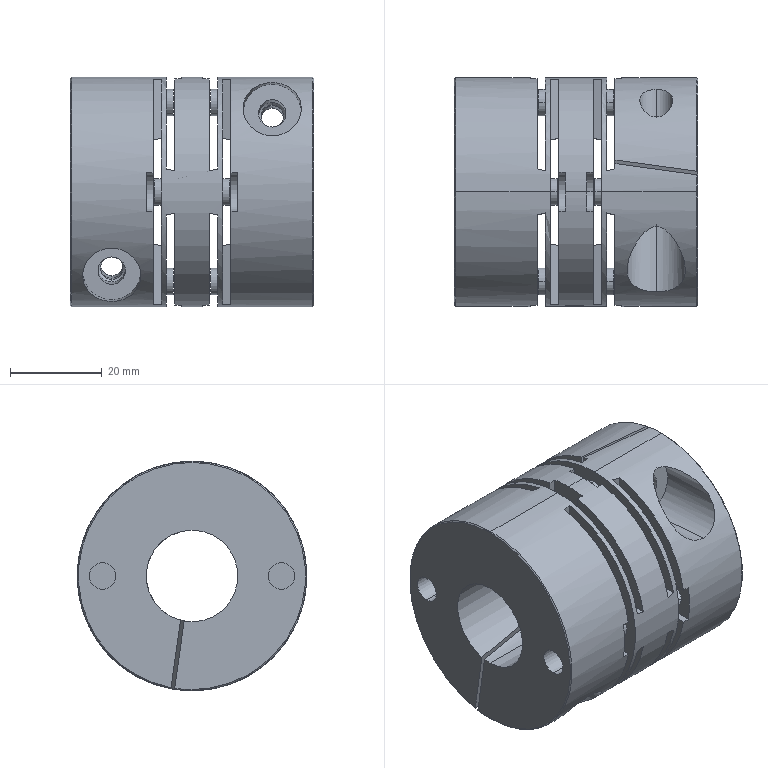Part | SolidWorks | features BaseBody 1 | 1 solid | 153 faces | box 53 x 50 x 50 mm | volume 68294 mm3 | plane 75 | cylinder 64 | cone 14 | commonest cylinder face diameters 5.8 x24 8.5 x10 4.917 x8 20 x6 6 x4 7.2 x4